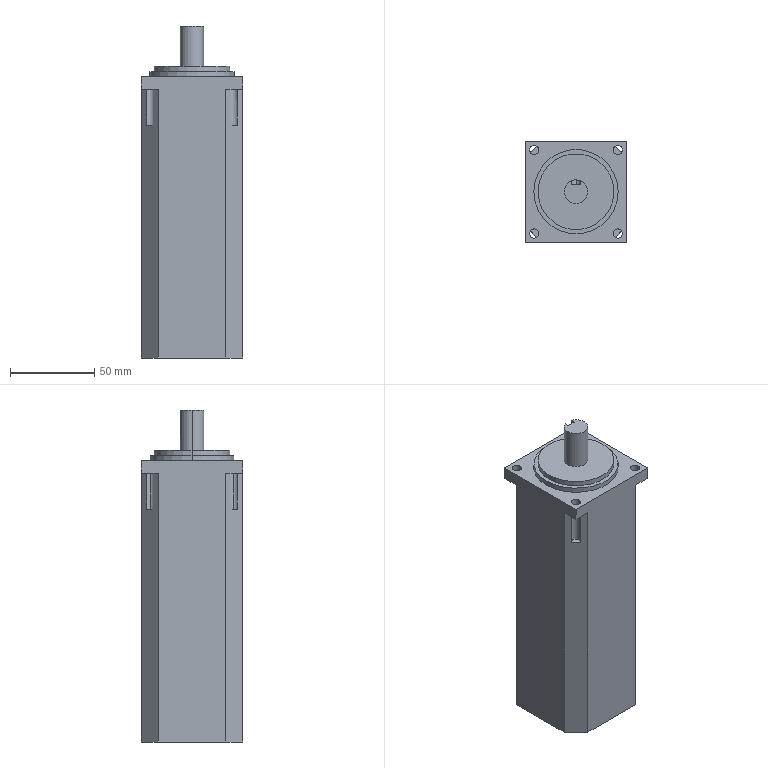Part | 1 solid | 985 faces | box 60 x 60 x 196.8 mm | volume 580879 mm3 | plane 696 | spline 273 | cylinder 16 | commonest cylinder face diameters 5.5 x8 5 x2 14 x2 45 x2 50 x2